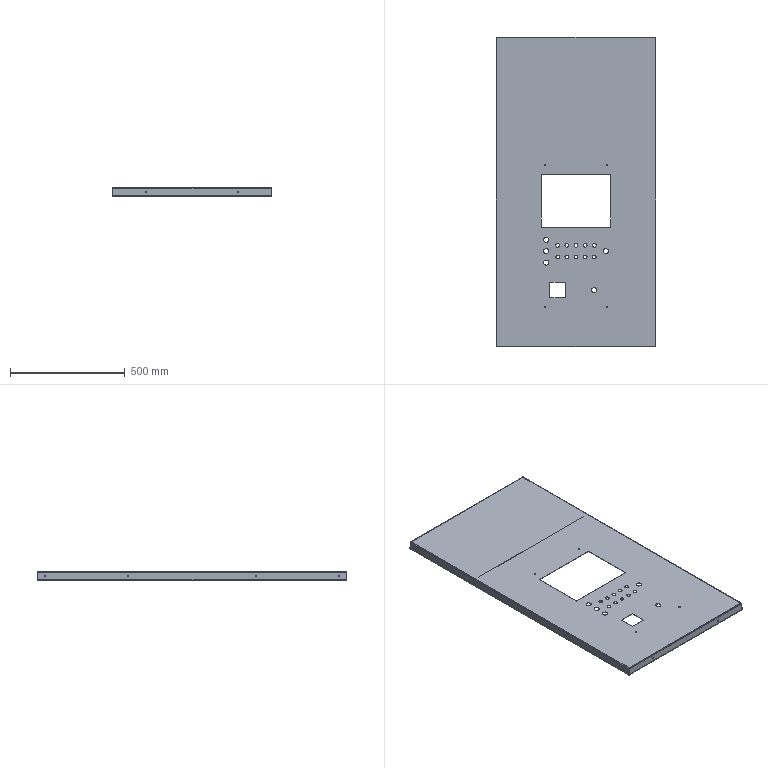Part | SolidWorks | features SMWeldBead 4, HoleWzd 3, EdgeFlange 2, BossThin 1, FlatPattern 1, ICE 1, SMBaseFlange 1, SheetMetal 1 | 1 solid | 189 faces | box 697 x 1351 x 38 mm | volume 1680620 mm3 | cylinder 82 | plane 67 | spline 40 | commonest cylinder face diameters 6.6 x24 16.2 x20 22 x10 4 x8 5.5 x8 7 x8